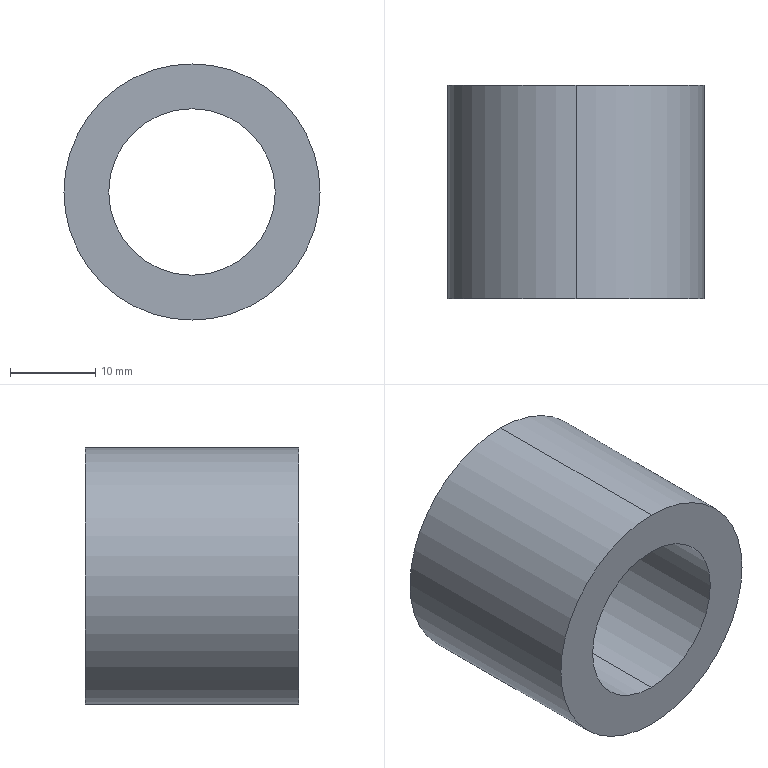Part | STEP file | 1 solid | 6 faces | box 30 x 25 x 30 mm | volume 10205 mm3 | cylinder 4 | plane 2 | commonest cylinder face diameters 19.5 x2 30 x2
STEP:
#1=CARTESIAN_POINT('',(0.,0.,0.));
#2=DIRECTION('',(0.,0.,1.));
#3=DIRECTION('',(1.,0.,0.));
#4=AXIS2_PLACEMENT_3D('',#1,#2,#3);
#5=CARTESIAN_POINT('',(0.,25.,-9.75));
#6=VERTEX_POINT('',#5);
#7=CARTESIAN_POINT('',(0.,0.,-9.75));
#8=VERTEX_POINT('',#7);
#9=CARTESIAN_POINT('',(0.,25.,-9.75));
#10=DIRECTION('',(0.,-1.,0.));
#11=VECTOR('',#10,1.);
#12=LINE('',#9,#11);
#13=CARTESIAN_POINT('',(0.,25.,0.));
#14=DIRECTION('',(0.,-1.,0.));
#15=DIRECTION('',(0.,0.,-1.));
#16=AXIS2_PLACEMENT_3D('',#13,#14,#15);
#17=CYLINDRICAL_SURFACE('',#16,9.75);
#18=CARTESIAN_POINT('',(6.283,0.));
#19=DIRECTION('',(0.,1.));
#20=VECTOR('',#19,1.);
#21=LINE('',#18,#20);
#22=(GEOMETRIC_REPRESENTATION_CONTEXT(2)PARAMETRIC_REPRESENTATION_CONTEXT()REPRESENTATION_CONTEXT('',''));
#23=DEFINITIONAL_REPRESENTATION('',(#21),#22);
#24=PCURVE('',#17,#23);
#25=CARTESIAN_POINT('',(0.,25.,0.));
#26=DIRECTION('',(0.,-1.,0.));
#27=DIRECTION('',(0.,0.,-1.));
#28=AXIS2_PLACEMENT_3D('',#25,#26,#27);
#29=CYLINDRICAL_SURFACE('',#28,9.75);
#30=CARTESIAN_POINT('',(0.,0.));
#31=DIRECTION('',(0.,1.));
#32=VECTOR('',#31,1.);
#33=LINE('',#30,#32);
#34=(GEOMETRIC_REPRESENTATION_CONTEXT(2)PARAMETRIC_REPRESENTATION_CONTEXT()REPRESENTATION_CONTEXT('',''));
#35=DEFINITIONAL_REPRESENTATION('',(#33),#34);
#36=PCURVE('',#29,#35);
#37=SURFACE_CURVE('',#12,(#24,#36),.PCURVE_S1.);
#38=EDGE_CURVE('',#6,#8,#37,.T.);
#39=ORIENTED_EDGE('',*,*,#38,.T.);
#40=CARTESIAN_POINT('',(0.,0.,9.75));
#41=VERTEX_POINT('',#40);
#42=CARTESIAN_POINT('',(0.,0.,0.));
#43=DIRECTION('',(0.,1.,0.));
#44=DIRECTION('',(0.,0.,1.));
#45=AXIS2_PLACEMENT_3D('',#42,#43,#44);
#46=CIRCLE('',#45,9.75);
#47=CARTESIAN_POINT('',(9.425,25.));
#48=DIRECTION('',(-1.,0.));
#49=VECTOR('',#48,1.);
#50=LINE('',#47,#49);
#51=(GEOMETRIC_REPRESENTATION_CONTEXT(2)PARAMETRIC_REPRESENTATION_CONTEXT()REPRESENTATION_CONTEXT('',''));
#52=DEFINITIONAL_REPRESENTATION('',(#50),#51);
#53=PCURVE('',#17,#52);
#54=CARTESIAN_POINT('',(0.,0.,0.));
#55=DIRECTION('',(0.,1.,0.));
#56=DIRECTION('',(0.,0.,1.));
#57=AXIS2_PLACEMENT_3D('',#54,#55,#56);
#58=PLANE('',#57);
#59=CARTESIAN_POINT('',(0.,0.));
#60=DIRECTION('',(1.,0.));
#61=AXIS2_PLACEMENT_2D('',#59,#60);
#62=CIRCLE('',#61,9.75);
#63=(GEOMETRIC_REPRESENTATION_CONTEXT(2)PARAMETRIC_REPRESENTATION_CONTEXT()REPRESENTATION_CONTEXT('',''));
#64=DEFINITIONAL_REPRESENTATION('',(#62),#63);
#65=PCURVE('',#58,#64);
#66=SURFACE_CURVE('',#46,(#53,#65),.PCURVE_S1.);
#67=EDGE_CURVE('',#8,#41,#66,.T.);
#68=ORIENTED_EDGE('',*,*,#67,.T.);
#69=CARTESIAN_POINT('',(0.,25.,9.75));
#70=VERTEX_POINT('',#69);
#71=CARTESIAN_POINT('',(0.,25.,9.75));
#72=DIRECTION('',(0.,-1.,0.));
#73=VECTOR('',#72,1.);
#74=LINE('',#71,#73);
#75=CARTESIAN_POINT('',(3.142,0.));
#76=DIRECTION('',(0.,1.));
#77=VECTOR('',#76,1.);
#78=LINE('',#75,#77);
#79=(GEOMETRIC_REPRESENTATION_CONTEXT(2)PARAMETRIC_REPRESENTATION_CONTEXT()REPRESENTATION_CONTEXT('',''));
#80=DEFINITIONAL_REPRESENTATION('',(#78),#79);
#81=PCURVE('',#17,#80);
#82=CARTESIAN_POINT('',(3.142,0.));
#83=DIRECTION('',(0.,1.));
#84=VECTOR('',#83,1.);
#85=LINE('',#82,#84);
#86=(GEOMETRIC_REPRESENTATION_CONTEXT(2)PARAMETRIC_REPRESENTATION_CONTEXT()REPRESENTATION_CONTEXT('',''));
#87=DEFINITIONAL_REPRESENTATION('',(#85),#86);
#88=PCURVE('',#29,#87);
#89=SURFACE_CURVE('',#74,(#81,#88),.PCURVE_S1.);
#90=EDGE_CURVE('',#70,#41,#89,.T.);
#91=ORIENTED_EDGE('',*,*,#90,.F.);
#92=CARTESIAN_POINT('',(0.,25.,0.));
#93=DIRECTION('',(0.,1.,0.));
#94=DIRECTION('',(0.,0.,1.));
#95=AXIS2_PLACEMENT_3D('',#92,#93,#94);
#96=CIRCLE('',#95,9.75);
#97=CARTESIAN_POINT('',(9.425,0.));
#98=DIRECTION('',(-1.,0.));
#99=VECTOR('',#98,1.);
#100=LINE('',#97,#99);
#101=(GEOMETRIC_REPRESENTATION_CONTEXT(2)PARAMETRIC_REPRESENTATION_CONTEXT()REPRESENTATION_CONTEXT('',''));
#102=DEFINITIONAL_REPRESENTATION('',(#100),#101);
#103=PCURVE('',#17,#102);
#104=CARTESIAN_POINT('',(0.,25.,0.));
#105=DIRECTION('',(0.,1.,0.));
#106=DIRECTION('',(0.,0.,1.));
#107=AXIS2_PLACEMENT_3D('',#104,#105,#106);
#108=PLANE('',#107);
#109=CARTESIAN_POINT('',(0.,0.));
#110=DIRECTION('',(1.,0.));
#111=AXIS2_PLACEMENT_2D('',#109,#110);
#112=CIRCLE('',#111,9.75);
#113=(GEOMETRIC_REPRESENTATION_CONTEXT(2)PARAMETRIC_REPRESENTATION_CONTEXT()REPRESENTATION_CONTEXT('',''));
#114=DEFINITIONAL_REPRESENTATION('',(#112),#113);
#115=PCURVE('',#108,#114);
#116=SURFACE_CURVE('',#96,(#103,#115),.PCURVE_S1.);
#117=EDGE_CURVE('',#6,#70,#116,.T.);
#118=ORIENTED_EDGE('',*,*,#117,.F.);
#119=EDGE_LOOP('',(#39,#68,#91,#118));
#120=FACE_BOUND('',#119,.F.);
#121=ADVANCED_FACE('',(#120),#17,.F.);
#122=CARTESIAN_POINT('',(0.,25.,15.));
#123=VERTEX_POINT('',#122);
#124=CARTESIAN_POINT('',(0.,25.,-15.));
#125=VERTEX_POINT('',#124);
#126=CARTESIAN_POINT('',(0.,25.,0.));
#127=DIRECTION('',(0.,1.,0.));
#128=DIRECTION('',(0.,0.,1.));
#129=AXIS2_PLACEMENT_3D('',#126,#127,#128);
#130=CIRCLE('',#129,15.);
#131=CARTESIAN_POINT('',(0.,25.,0.));
#132=DIRECTION('',(0.,-1.,0.));
#133=DIRECTION('',(0.,0.,-1.));
#134=AXIS2_PLACEMENT_3D('',#131,#132,#133);
#135=CYLINDRICAL_SURFACE('',#134,15.);
#136=CARTESIAN_POINT('',(3.142,0.));
#137=DIRECTION('',(-1.,0.));
#138=VECTOR('',#137,1.);
#139=LINE('',#136,#138);
#140=(GEOMETRIC_REPRESENTATION_CONTEXT(2)PARAMETRIC_REPRESENTATION_CONTEXT()REPRESENTATION_CONTEXT('',''));
#141=DEFINITIONAL_REPRESENTATION('',(#139),#140);
#142=PCURVE('',#135,#141);
#143=CARTESIAN_POINT('',(0.,0.));
#144=DIRECTION('',(1.,0.));
#145=AXIS2_PLACEMENT_2D('',#143,#144);
#146=CIRCLE('',#145,15.);
#147=(GEOMETRIC_REPRESENTATION_CONTEXT(2)PARAMETRIC_REPRESENTATION_CONTEXT()REPRESENTATION_CONTEXT('',''));
#148=DEFINITIONAL_REPRESENTATION('',(#146),#147);
#149=PCURVE('',#108,#148);
#150=SURFACE_CURVE('',#130,(#142,#149),.PCURVE_S1.);
#151=EDGE_CURVE('',#123,#125,#150,.T.);
#152=ORIENTED_EDGE('',*,*,#151,.F.);
#153=CARTESIAN_POINT('',(0.,0.,15.));
#154=VERTEX_POINT('',#153);
#155=CARTESIAN_POINT('',(0.,25.,15.));
#156=DIRECTION('',(0.,-1.,0.));
#157=VECTOR('',#156,1.);
#158=LINE('',#155,#157);
#159=CARTESIAN_POINT('',(3.142,0.));
#160=DIRECTION('',(0.,1.));
#161=VECTOR('',#160,1.);
#162=LINE('',#159,#161);
#163=(GEOMETRIC_REPRESENTATION_CONTEXT(2)PARAMETRIC_REPRESENTATION_CONTEXT()REPRESENTATION_CONTEXT('',''));
#164=DEFINITIONAL_REPRESENTATION('',(#162),#163);
#165=PCURVE('',#135,#164);
#166=CARTESIAN_POINT('',(0.,25.,0.));
#167=DIRECTION('',(0.,-1.,0.));
#168=DIRECTION('',(0.,0.,-1.));
#169=AXIS2_PLACEMENT_3D('',#166,#167,#168);
#170=CYLINDRICAL_SURFACE('',#169,15.);
#171=CARTESIAN_POINT('',(3.142,0.));
#172=DIRECTION('',(0.,1.));
#173=VECTOR('',#172,1.);
#174=LINE('',#171,#173);
#175=(GEOMETRIC_REPRESENTATION_CONTEXT(2)PARAMETRIC_REPRESENTATION_CONTEXT()REPRESENTATION_CONTEXT('',''));
#176=DEFINITIONAL_REPRESENTATION('',(#174),#175);
#177=PCURVE('',#170,#176);
#178=SURFACE_CURVE('',#158,(#165,#177),.PCURVE_S1.);
#179=EDGE_CURVE('',#123,#154,#178,.T.);
#180=ORIENTED_EDGE('',*,*,#179,.T.);
#181=CARTESIAN_POINT('',(0.,0.,-15.));
#182=VERTEX_POINT('',#181);
#183=CARTESIAN_POINT('',(0.,0.,0.));
#184=DIRECTION('',(0.,1.,0.));
#185=DIRECTION('',(0.,0.,1.));
#186=AXIS2_PLACEMENT_3D('',#183,#184,#185);
#187=CIRCLE('',#186,15.);
#188=CARTESIAN_POINT('',(3.142,25.));
#189=DIRECTION('',(-1.,0.));
#190=VECTOR('',#189,1.);
#191=LINE('',#188,#190);
#192=(GEOMETRIC_REPRESENTATION_CONTEXT(2)PARAMETRIC_REPRESENTATION_CONTEXT()REPRESENTATION_CONTEXT('',''));
#193=DEFINITIONAL_REPRESENTATION('',(#191),#192);
#194=PCURVE('',#135,#193);
#195=CARTESIAN_POINT('',(0.,0.));
#196=DIRECTION('',(1.,0.));
#197=AXIS2_PLACEMENT_2D('',#195,#196);
#198=CIRCLE('',#197,15.);
#199=(GEOMETRIC_REPRESENTATION_CONTEXT(2)PARAMETRIC_REPRESENTATION_CONTEXT()REPRESENTATION_CONTEXT('',''));
#200=DEFINITIONAL_REPRESENTATION('',(#198),#199);
#201=PCURVE('',#58,#200);
#202=SURFACE_CURVE('',#187,(#194,#201),.PCURVE_S1.);
#203=EDGE_CURVE('',#154,#182,#202,.T.);
#204=ORIENTED_EDGE('',*,*,#203,.T.);
#205=CARTESIAN_POINT('',(0.,25.,-15.));
#206=DIRECTION('',(0.,-1.,0.));
#207=VECTOR('',#206,1.);
#208=LINE('',#205,#207);
#209=CARTESIAN_POINT('',(0.,0.));
#210=DIRECTION('',(0.,1.));
#211=VECTOR('',#210,1.);
#212=LINE('',#209,#211);
#213=(GEOMETRIC_REPRESENTATION_CONTEXT(2)PARAMETRIC_REPRESENTATION_CONTEXT()REPRESENTATION_CONTEXT('',''));
#214=DEFINITIONAL_REPRESENTATION('',(#212),#213);
#215=PCURVE('',#135,#214);
#216=CARTESIAN_POINT('',(6.283,0.));
#217=DIRECTION('',(0.,1.));
#218=VECTOR('',#217,1.);
#219=LINE('',#216,#218);
#220=(GEOMETRIC_REPRESENTATION_CONTEXT(2)PARAMETRIC_REPRESENTATION_CONTEXT()REPRESENTATION_CONTEXT('',''));
#221=DEFINITIONAL_REPRESENTATION('',(#219),#220);
#222=PCURVE('',#170,#221);
#223=SURFACE_CURVE('',#208,(#215,#222),.PCURVE_S1.);
#224=EDGE_CURVE('',#125,#182,#223,.T.);
#225=ORIENTED_EDGE('',*,*,#224,.F.);
#226=EDGE_LOOP('',(#152,#180,#204,#225));
#227=FACE_BOUND('',#226,.T.);
#228=ADVANCED_FACE('',(#227),#135,.T.);
#229=CARTESIAN_POINT('',(0.,25.,0.));
#230=DIRECTION('',(0.,1.,0.));
#231=DIRECTION('',(0.,0.,1.));
#232=AXIS2_PLACEMENT_3D('',#229,#230,#231);
#233=CIRCLE('',#232,15.);
#234=CARTESIAN_POINT('',(0.,0.));
#235=DIRECTION('',(1.,0.));
#236=AXIS2_PLACEMENT_2D('',#234,#235);
#237=CIRCLE('',#236,15.);
#238=(GEOMETRIC_REPRESENTATION_CONTEXT(2)PARAMETRIC_REPRESENTATION_CONTEXT()REPRESENTATION_CONTEXT('',''));
#239=DEFINITIONAL_REPRESENTATION('',(#237),#238);
#240=PCURVE('',#108,#239);
#241=CARTESIAN_POINT('',(9.425,0.));
#242=DIRECTION('',(-1.,0.));
#243=VECTOR('',#242,1.);
#244=LINE('',#241,#243);
#245=(GEOMETRIC_REPRESENTATION_CONTEXT(2)PARAMETRIC_REPRESENTATION_CONTEXT()REPRESENTATION_CONTEXT('',''));
#246=DEFINITIONAL_REPRESENTATION('',(#244),#245);
#247=PCURVE('',#170,#246);
#248=SURFACE_CURVE('',#233,(#240,#247),.PCURVE_S1.);
#249=EDGE_CURVE('',#125,#123,#248,.T.);
#250=ORIENTED_EDGE('',*,*,#249,.T.);
#251=ORIENTED_EDGE('',*,*,#151,.T.);
#252=EDGE_LOOP('',(#250,#251));
#253=FACE_BOUND('',#252,.T.);
#254=ORIENTED_EDGE('',*,*,#117,.F.);
#255=CARTESIAN_POINT('',(0.,25.,0.));
#256=DIRECTION('',(0.,1.,0.));
#257=DIRECTION('',(0.,0.,1.));
#258=AXIS2_PLACEMENT_3D('',#255,#256,#257);
#259=CIRCLE('',#258,9.75);
#260=CARTESIAN_POINT('',(0.,0.));
#261=DIRECTION('',(1.,0.));
#262=AXIS2_PLACEMENT_2D('',#260,#261);
#263=CIRCLE('',#262,9.75);
#264=(GEOMETRIC_REPRESENTATION_CONTEXT(2)PARAMETRIC_REPRESENTATION_CONTEXT()REPRESENTATION_CONTEXT('',''));
#265=DEFINITIONAL_REPRESENTATION('',(#263),#264);
#266=PCURVE('',#108,#265);
#267=CARTESIAN_POINT('',(3.142,0.));
#268=DIRECTION('',(-1.,0.));
#269=VECTOR('',#268,1.);
#270=LINE('',#267,#269);
#271=(GEOMETRIC_REPRESENTATION_CONTEXT(2)PARAMETRIC_REPRESENTATION_CONTEXT()REPRESENTATION_CONTEXT('',''));
#272=DEFINITIONAL_REPRESENTATION('',(#270),#271);
#273=PCURVE('',#29,#272);
#274=SURFACE_CURVE('',#259,(#266,#273),.PCURVE_S1.);
#275=EDGE_CURVE('',#70,#6,#274,.T.);
#276=ORIENTED_EDGE('',*,*,#275,.F.);
#277=EDGE_LOOP('',(#254,#276));
#278=FACE_BOUND('',#277,.T.);
#279=ADVANCED_FACE('',(#253,#278),#108,.T.);
#280=CARTESIAN_POINT('',(0.,0.,0.));
#281=DIRECTION('',(0.,1.,0.));
#282=DIRECTION('',(0.,0.,1.));
#283=AXIS2_PLACEMENT_3D('',#280,#281,#282);
#284=CIRCLE('',#283,15.);
#285=CARTESIAN_POINT('',(0.,0.));
#286=DIRECTION('',(1.,0.));
#287=AXIS2_PLACEMENT_2D('',#285,#286);
#288=CIRCLE('',#287,15.);
#289=(GEOMETRIC_REPRESENTATION_CONTEXT(2)PARAMETRIC_REPRESENTATION_CONTEXT()REPRESENTATION_CONTEXT('',''));
#290=DEFINITIONAL_REPRESENTATION('',(#288),#289);
#291=PCURVE('',#58,#290);
#292=CARTESIAN_POINT('',(9.425,25.));
#293=DIRECTION('',(-1.,0.));
#294=VECTOR('',#293,1.);
#295=LINE('',#292,#294);
#296=(GEOMETRIC_REPRESENTATION_CONTEXT(2)PARAMETRIC_REPRESENTATION_CONTEXT()REPRESENTATION_CONTEXT('',''));
#297=DEFINITIONAL_REPRESENTATION('',(#295),#296);
#298=PCURVE('',#170,#297);
#299=SURFACE_CURVE('',#284,(#291,#298),.PCURVE_S1.);
#300=EDGE_CURVE('',#182,#154,#299,.T.);
#301=ORIENTED_EDGE('',*,*,#300,.F.);
#302=ORIENTED_EDGE('',*,*,#203,.F.);
#303=EDGE_LOOP('',(#301,#302));
#304=FACE_BOUND('',#303,.T.);
#305=ORIENTED_EDGE('',*,*,#67,.T.);
#306=CARTESIAN_POINT('',(0.,0.,0.));
#307=DIRECTION('',(0.,1.,0.));
#308=DIRECTION('',(0.,0.,1.));
#309=AXIS2_PLACEMENT_3D('',#306,#307,#308);
#310=CIRCLE('',#309,9.75);
#311=CARTESIAN_POINT('',(0.,0.));
#312=DIRECTION('',(1.,0.));
#313=AXIS2_PLACEMENT_2D('',#311,#312);
#314=CIRCLE('',#313,9.75);
#315=(GEOMETRIC_REPRESENTATION_CONTEXT(2)PARAMETRIC_REPRESENTATION_CONTEXT()REPRESENTATION_CONTEXT('',''));
#316=DEFINITIONAL_REPRESENTATION('',(#314),#315);
#317=PCURVE('',#58,#316);
#318=CARTESIAN_POINT('',(3.142,25.));
#319=DIRECTION('',(-1.,0.));
#320=VECTOR('',#319,1.);
#321=LINE('',#318,#320);
#322=(GEOMETRIC_REPRESENTATION_CONTEXT(2)PARAMETRIC_REPRESENTATION_CONTEXT()REPRESENTATION_CONTEXT('',''));
#323=DEFINITIONAL_REPRESENTATION('',(#321),#322);
#324=PCURVE('',#29,#323);
#325=SURFACE_CURVE('',#310,(#317,#324),.PCURVE_S1.);
#326=EDGE_CURVE('',#41,#8,#325,.T.);
#327=ORIENTED_EDGE('',*,*,#326,.T.);
#328=EDGE_LOOP('',(#305,#327));
#329=FACE_BOUND('',#328,.T.);
#330=ADVANCED_FACE('',(#304,#329),#58,.F.);
#331=ORIENTED_EDGE('',*,*,#179,.F.);
#332=ORIENTED_EDGE('',*,*,#249,.F.);
#333=ORIENTED_EDGE('',*,*,#224,.T.);
#334=ORIENTED_EDGE('',*,*,#300,.T.);
#335=EDGE_LOOP('',(#331,#332,#333,#334));
#336=FACE_BOUND('',#335,.T.);
#337=ADVANCED_FACE('',(#336),#170,.T.);
#338=ORIENTED_EDGE('',*,*,#326,.T.);
#339=ORIENTED_EDGE('',*,*,#38,.F.);
#340=ORIENTED_EDGE('',*,*,#275,.F.);
#341=ORIENTED_EDGE('',*,*,#90,.T.);
#342=EDGE_LOOP('',(#338,#339,#340,#341));
#343=FACE_BOUND('',#342,.F.);
#344=ADVANCED_FACE('',(#343),#29,.F.);
#345=CLOSED_SHELL('',(#121,#228,#279,#330,#337,#344));
#346=MANIFOLD_SOLID_BREP('',#345);
#347=(LENGTH_UNIT()NAMED_UNIT(*)SI_UNIT(.MILLI.,.METRE.));
#348=UNCERTAINTY_MEASURE_WITH_UNIT(LENGTH_MEASURE(0.0000001),#347,'','');
#349=(NAMED_UNIT(*)PLANE_ANGLE_UNIT()SI_UNIT($,.RADIAN.));
#350=(NAMED_UNIT(*)SI_UNIT($,.STERADIAN.)SOLID_ANGLE_UNIT());
#351=(GEOMETRIC_REPRESENTATION_CONTEXT(3)GLOBAL_UNCERTAINTY_ASSIGNED_CONTEXT((#348))GLOBAL_UNIT_ASSIGNED_CONTEXT((#347,#349,#350))REPRESENTATION_CONTEXT('',''));
#352=ADVANCED_BREP_SHAPE_REPRESENTATION('',(#4,#346),#351);